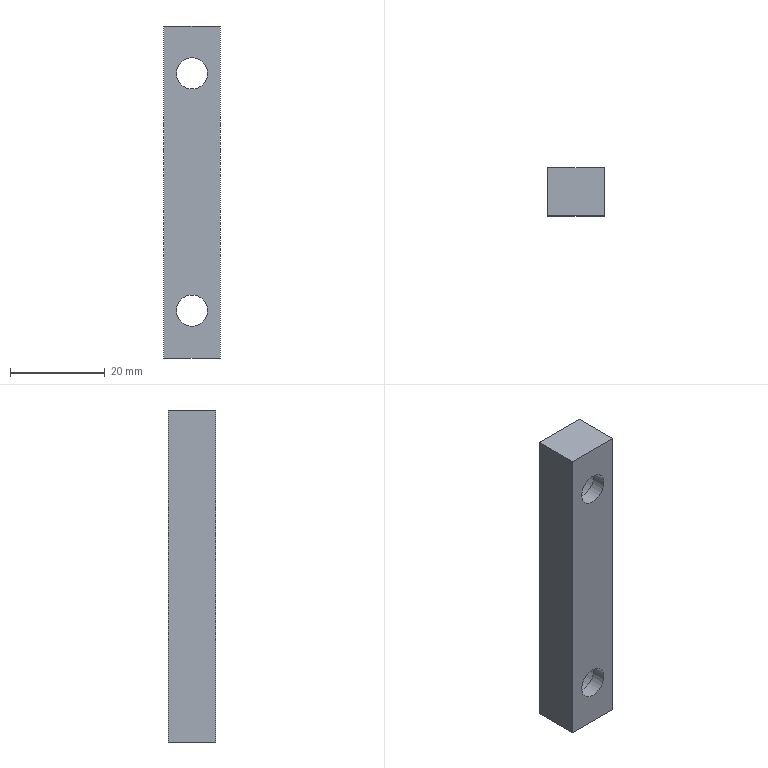Part | STEP file | solid 57 | 1 solid | 12 faces | box 12 x 10 x 70 mm | volume 6864 mm3 | plane 8 | cylinder 4 | commonest cylinder face diameters 6.6 x2 11 x2